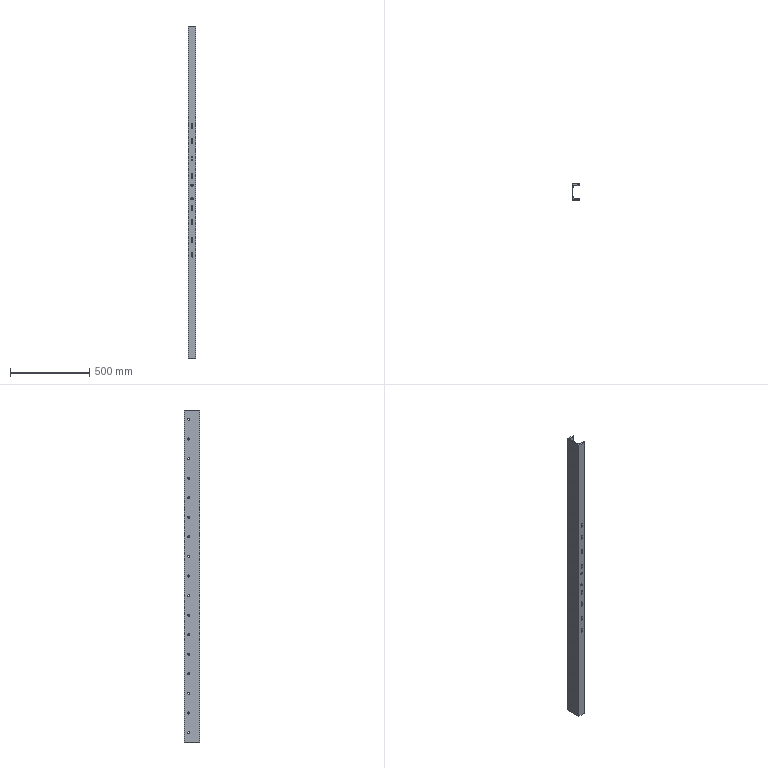Part | SolidWorks | features ICE 2, Extrusion 1 | 1 solid | 92 faces | box 50 x 100 x 2100 mm | volume 2750489 mm3 | cylinder 66 | plane 26 | commonest cylinder face diameters 13 x38 10.5 x24 9 x2 17 x2